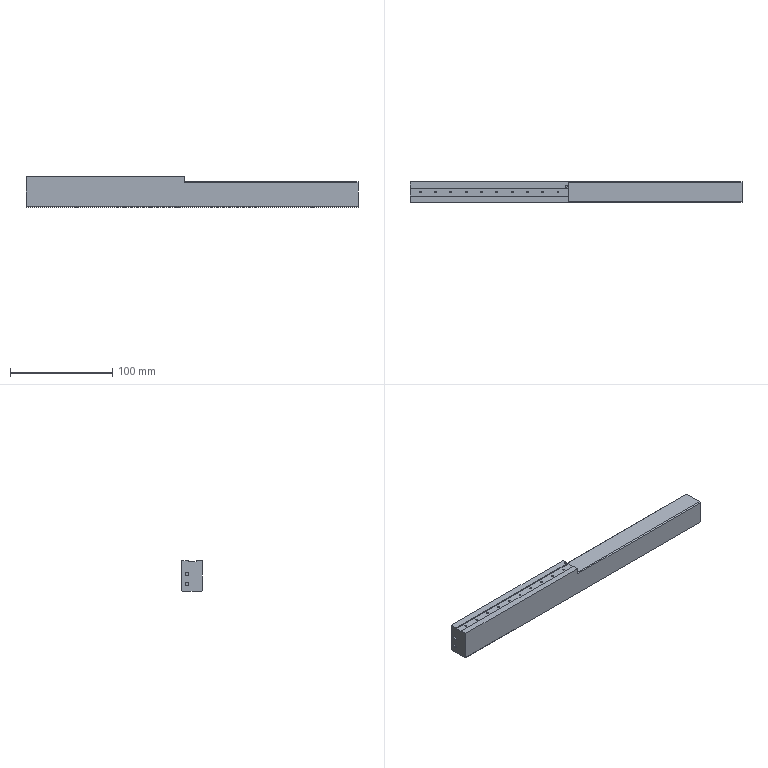Part | 1 solid | 97 faces | box 325 x 20 x 30 mm | volume 174943 mm3 | cylinder 54 | plane 43 | commonest cylinder face diameters 1.7 x22 2.5 x20 3.3 x12